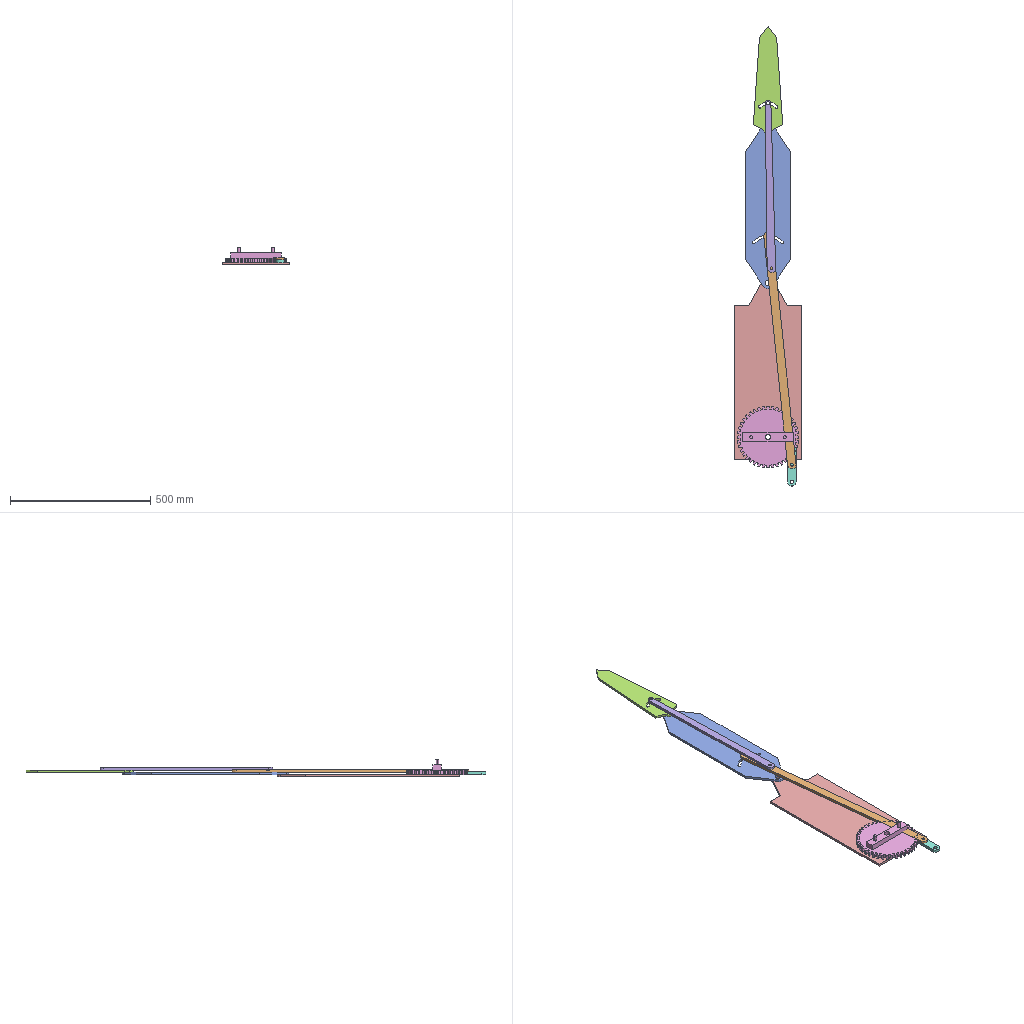Assembly | SolidWorks | 7 different items | 7 placed | box 240 x 1642 x 63 mm
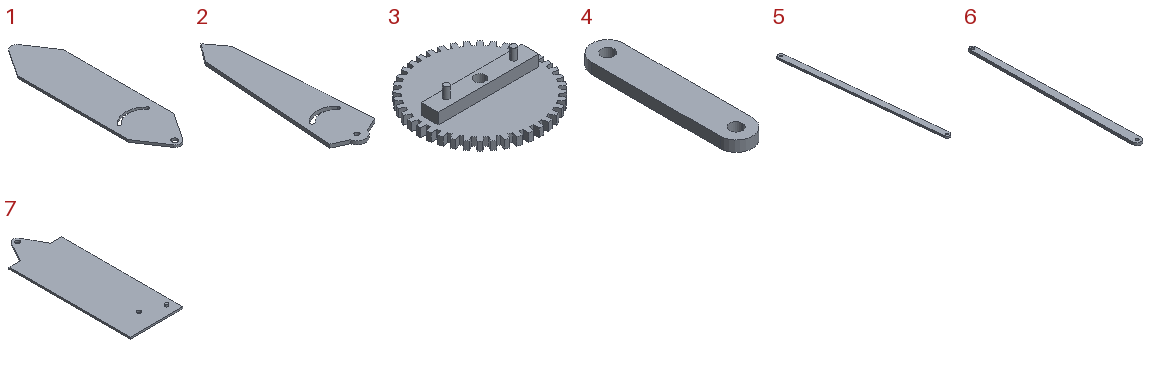Parts list (item | quantity | size | volume | features):
1 | x1 | 160 x 594 x 8 mm | 632396 mm3 | features Cut 1, Extrusion 1
2 | x1 | 105.1 x 383.944 x 8 mm | 223880 mm3 | features Cut 1, Extrusion 1
3 | x1 | 220 x 220 x 55 mm | 621975 mm3 | features ICE 2, Extrusion 1
4 | x1 | 30 x 149.604 x 10 mm | 40688 mm3 | features Extrusion 1
5 | x1 | 115.162 x 846.43 x 10 mm | 253110 mm3 | features Extrusion 1
6 | x1 | 37.197 x 615.099 x 10 mm | 152379 mm3 | features Extrusion 1
7 | x1 | 240 x 651.329 x 18 mm | 1117831 mm3 | features Extrusion 1, ICE 1
Mates (type | each side: item.copy, entity, surface, feature):
InPlace | 7.1 face plane Boss-Extrude1 | 1.1 plane
InPlace | 1.1 face plane Boss-Extrude1 | 2.1 plane
InPlace | 7.1 face plane Boss-Extrude1 | 3.1 plane
InPlace | 7.1 face plane Boss-Extrude2 | 4.1 plane
InPlace | 1.1 face plane Boss-Extrude1 | 5.1 plane
InPlace | 2.1 face plane Boss-Extrude1 | 6.1 plane